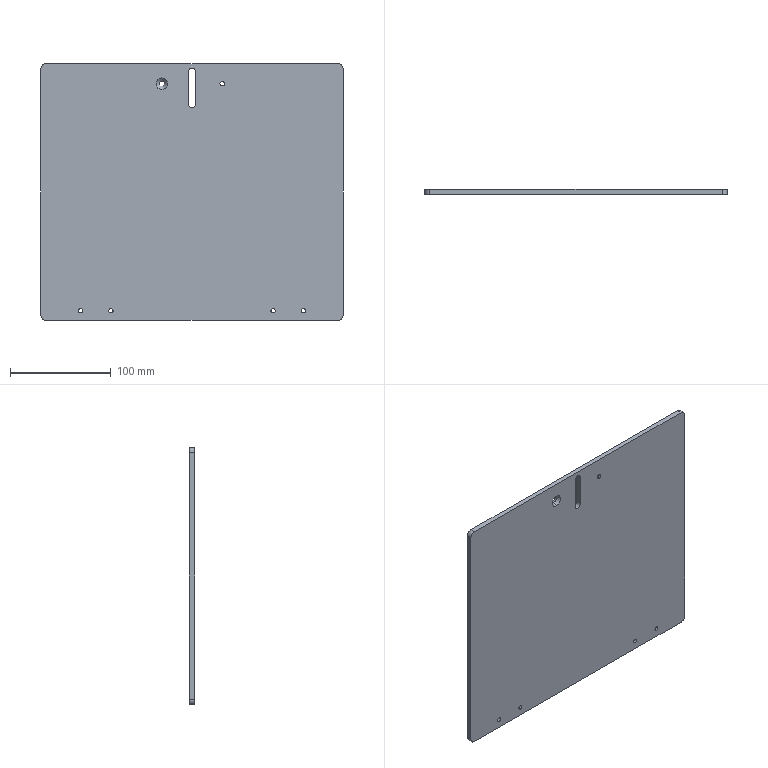Part | STEP file | H_ND24021-01-JG-032-SL | 1 solid | 31 faces | box 300 x 5 x 255 mm | volume 380407 mm3 | cylinder 19 | plane 8 | cone 4 | commonest cylinder face diameters 4.2 x8 10 x4 7 x3 4.5 x2 5.5 x2